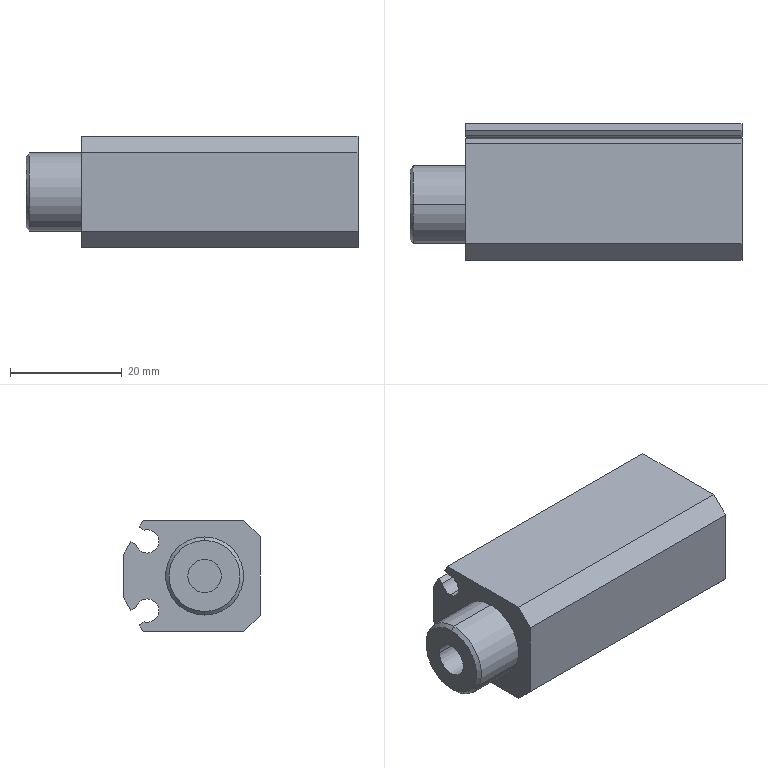Part | SolidWorks | features RefAxis 18, 3DProfileFeature 6, RevCut 3, Extrusion 1, Revolution 1 | 1 solid | 45 faces | box 59.5 x 24.5 x 20 mm | volume 16440 mm3 | plane 19 | cylinder 16 | cone 10 | commonest cylinder face diameters 4.2 x6 4.134 x4 6 x2 14 x2 16 x2
STEP:
#1=CARTESIAN_POINT('',(42.,7.258,0.));
#2=VERTEX_POINT('',#1);
#3=CARTESIAN_POINT('',(42.,8.5,2.067));
#4=VERTEX_POINT('',#3);
#5=CARTESIAN_POINT('',(42.,7.258,0.));
#6=DIRECTION('',(0.,0.515,0.8572));
#7=VECTOR('',#6,1000.);
#8=LINE('',#5,#7);
#9=EDGE_CURVE('',#2,#4,#8,.T.);
#10=ORIENTED_EDGE('',*,*,#9,.F.);
#11=CARTESIAN_POINT('',(42.,8.5,-2.067));
#12=VERTEX_POINT('',#11);
#13=CARTESIAN_POINT('',(42.,7.258,0.));
#14=DIRECTION('',(0.,0.515,-0.8572));
#15=VECTOR('',#14,1000.);
#16=LINE('',#13,#15);
#17=EDGE_CURVE('',#2,#12,#16,.T.);
#18=ORIENTED_EDGE('',*,*,#17,.T.);
#19=CARTESIAN_POINT('',(42.,8.5,0.));
#20=DIRECTION('',(0.,-1.,0.));
#21=DIRECTION('',(0.,0.,-1.));
#22=AXIS2_PLACEMENT_3D('',#19,#20,#21);
#23=CIRCLE('',#22,2.067);
#24=EDGE_CURVE('',#4,#12,#23,.T.);
#25=ORIENTED_EDGE('',*,*,#24,.F.);
#26=EDGE_LOOP('',(#10,#18,#25));
#27=FACE_OUTER_BOUND('',#26,.T.);
#28=CARTESIAN_POINT('',(42.,1007.258,0.));
#29=DIRECTION('',(0.,1.,0.));
#30=DIRECTION('',(0.,0.,1.));
#31=AXIS2_PLACEMENT_3D('',#28,#29,#30);
#32=CONICAL_SURFACE('',#31,1664.279,1.03);
#33=ADVANCED_FACE('',(#27),#32,.F.);
#34=CARTESIAN_POINT('',(42.,14.067,2.067));
#35=VERTEX_POINT('',#34);
#36=CARTESIAN_POINT('',(42.,14.067,-2.067));
#37=VERTEX_POINT('',#36);
#38=CARTESIAN_POINT('',(42.,14.067,0.));
#39=DIRECTION('',(0.,-1.,0.));
#40=DIRECTION('',(0.,0.,-1.));
#41=AXIS2_PLACEMENT_3D('',#38,#39,#40);
#42=CIRCLE('',#41,2.067);
#43=EDGE_CURVE('',#35,#37,#42,.T.);
#44=ORIENTED_EDGE('',*,*,#43,.F.);
#45=CARTESIAN_POINT('',(42.,7.258,2.067));
#46=DIRECTION('',(0.,-1.,0.));
#47=VECTOR('',#46,1000.);
#48=LINE('',#45,#47);
#49=EDGE_CURVE('',#35,#4,#48,.T.);
#50=ORIENTED_EDGE('',*,*,#49,.T.);
#51=ORIENTED_EDGE('',*,*,#24,.T.);
#52=CARTESIAN_POINT('',(42.,7.258,-2.067));
#53=DIRECTION('',(0.,-1.,0.));
#54=VECTOR('',#53,1000.);
#55=LINE('',#52,#54);
#56=EDGE_CURVE('',#37,#12,#55,.T.);
#57=ORIENTED_EDGE('',*,*,#56,.F.);
#58=EDGE_LOOP('',(#44,#50,#51,#57));
#59=FACE_OUTER_BOUND('',#58,.T.);
#60=CARTESIAN_POINT('',(42.,7.258,0.));
#61=DIRECTION('',(0.,-1.,0.));
#62=DIRECTION('',(0.,0.,-1.));
#63=AXIS2_PLACEMENT_3D('',#60,#61,#62);
#64=CYLINDRICAL_SURFACE('',#63,2.067);
#65=ADVANCED_FACE('',(#59),#64,.F.);
#66=ORIENTED_EDGE('',*,*,#43,.T.);
#67=CARTESIAN_POINT('',(42.,14.5,-2.5));
#68=VERTEX_POINT('',#67);
#69=CARTESIAN_POINT('',(42.,14.067,-2.067));
#70=DIRECTION('',(0.,0.7071,-0.7071));
#71=VECTOR('',#70,1000.);
#72=LINE('',#69,#71);
#73=EDGE_CURVE('',#37,#68,#72,.T.);
#74=ORIENTED_EDGE('',*,*,#73,.T.);
#75=CARTESIAN_POINT('',(42.,14.5,2.5));
#76=VERTEX_POINT('',#75);
#77=CARTESIAN_POINT('',(42.,14.5,0.));
#78=DIRECTION('',(0.,-1.,0.));
#79=DIRECTION('',(0.,0.,-1.));
#80=AXIS2_PLACEMENT_3D('',#77,#78,#79);
#81=CIRCLE('',#80,2.5);
#82=EDGE_CURVE('',#76,#68,#81,.T.);
#83=ORIENTED_EDGE('',*,*,#82,.F.);
#84=CARTESIAN_POINT('',(42.,14.067,2.067));
#85=DIRECTION('',(0.,0.7071,0.7071));
#86=VECTOR('',#85,1000.);
#87=LINE('',#84,#86);
#88=EDGE_CURVE('',#35,#76,#87,.T.);
#89=ORIENTED_EDGE('',*,*,#88,.F.);
#90=EDGE_LOOP('',(#66,#74,#83,#89));
#91=FACE_OUTER_BOUND('',#90,.T.);
#92=CARTESIAN_POINT('',(42.,14.067,0.));
#93=DIRECTION('',(0.,1.,0.));
#94=DIRECTION('',(0.,0.,1.));
#95=AXIS2_PLACEMENT_3D('',#92,#93,#94);
#96=CONICAL_SURFACE('',#95,2.067,0.7854);
#97=ADVANCED_FACE('',(#91),#96,.F.);
#98=CARTESIAN_POINT('',(6.5,7.258,0.));
#99=VERTEX_POINT('',#98);
#100=CARTESIAN_POINT('',(6.5,8.5,2.067));
#101=VERTEX_POINT('',#100);
#102=CARTESIAN_POINT('',(6.5,7.258,0.));
#103=DIRECTION('',(0.,0.515,0.8572));
#104=VECTOR('',#103,1000.);
#105=LINE('',#102,#104);
#106=EDGE_CURVE('',#99,#101,#105,.T.);
#107=ORIENTED_EDGE('',*,*,#106,.F.);
#108=CARTESIAN_POINT('',(6.5,8.5,-2.067));
#109=VERTEX_POINT('',#108);
#110=CARTESIAN_POINT('',(6.5,7.258,0.));
#111=DIRECTION('',(0.,0.515,-0.8572));
#112=VECTOR('',#111,1000.);
#113=LINE('',#110,#112);
#114=EDGE_CURVE('',#99,#109,#113,.T.);
#115=ORIENTED_EDGE('',*,*,#114,.T.);
#116=CARTESIAN_POINT('',(6.5,8.5,0.));
#117=DIRECTION('',(0.,-1.,0.));
#118=DIRECTION('',(0.,0.,-1.));
#119=AXIS2_PLACEMENT_3D('',#116,#117,#118);
#120=CIRCLE('',#119,2.067);
#121=EDGE_CURVE('',#101,#109,#120,.T.);
#122=ORIENTED_EDGE('',*,*,#121,.F.);
#123=EDGE_LOOP('',(#107,#115,#122));
#124=FACE_OUTER_BOUND('',#123,.T.);
#125=CARTESIAN_POINT('',(6.5,1007.258,0.));
#126=DIRECTION('',(0.,1.,0.));
#127=DIRECTION('',(0.,0.,1.));
#128=AXIS2_PLACEMENT_3D('',#125,#126,#127);
#129=CONICAL_SURFACE('',#128,1664.279,1.03);
#130=ADVANCED_FACE('',(#124),#129,.F.);
#131=CARTESIAN_POINT('',(6.5,14.067,2.067));
#132=VERTEX_POINT('',#131);
#133=CARTESIAN_POINT('',(6.5,14.067,-2.067));
#134=VERTEX_POINT('',#133);
#135=CARTESIAN_POINT('',(6.5,14.067,0.));
#136=DIRECTION('',(0.,-1.,0.));
#137=DIRECTION('',(0.,0.,-1.));
#138=AXIS2_PLACEMENT_3D('',#135,#136,#137);
#139=CIRCLE('',#138,2.067);
#140=EDGE_CURVE('',#132,#134,#139,.T.);
#141=ORIENTED_EDGE('',*,*,#140,.F.);
#142=CARTESIAN_POINT('',(6.5,7.258,2.067));
#143=DIRECTION('',(0.,-1.,0.));
#144=VECTOR('',#143,1000.);
#145=LINE('',#142,#144);
#146=EDGE_CURVE('',#132,#101,#145,.T.);
#147=ORIENTED_EDGE('',*,*,#146,.T.);
#148=ORIENTED_EDGE('',*,*,#121,.T.);
#149=CARTESIAN_POINT('',(6.5,7.258,-2.067));
#150=DIRECTION('',(0.,-1.,0.));
#151=VECTOR('',#150,1000.);
#152=LINE('',#149,#151);
#153=EDGE_CURVE('',#134,#109,#152,.T.);
#154=ORIENTED_EDGE('',*,*,#153,.F.);
#155=EDGE_LOOP('',(#141,#147,#148,#154));
#156=FACE_OUTER_BOUND('',#155,.T.);
#157=CARTESIAN_POINT('',(6.5,7.258,0.));
#158=DIRECTION('',(0.,-1.,0.));
#159=DIRECTION('',(0.,0.,-1.));
#160=AXIS2_PLACEMENT_3D('',#157,#158,#159);
#161=CYLINDRICAL_SURFACE('',#160,2.067);
#162=ADVANCED_FACE('',(#156),#161,.F.);
#163=ORIENTED_EDGE('',*,*,#140,.T.);
#164=CARTESIAN_POINT('',(6.5,14.5,-2.5));
#165=VERTEX_POINT('',#164);
#166=CARTESIAN_POINT('',(6.5,14.067,-2.067));
#167=DIRECTION('',(0.,0.7071,-0.7071));
#168=VECTOR('',#167,1000.);
#169=LINE('',#166,#168);
#170=EDGE_CURVE('',#134,#165,#169,.T.);
#171=ORIENTED_EDGE('',*,*,#170,.T.);
#172=CARTESIAN_POINT('',(6.5,14.5,2.5));
#173=VERTEX_POINT('',#172);
#174=CARTESIAN_POINT('',(6.5,14.5,0.));
#175=DIRECTION('',(0.,-1.,0.));
#176=DIRECTION('',(0.,0.,-1.));
#177=AXIS2_PLACEMENT_3D('',#174,#175,#176);
#178=CIRCLE('',#177,2.5);
#179=EDGE_CURVE('',#173,#165,#178,.T.);
#180=ORIENTED_EDGE('',*,*,#179,.F.);
#181=CARTESIAN_POINT('',(6.5,14.067,2.067));
#182=DIRECTION('',(0.,0.7071,0.7071));
#183=VECTOR('',#182,1000.);
#184=LINE('',#181,#183);
#185=EDGE_CURVE('',#132,#173,#184,.T.);
#186=ORIENTED_EDGE('',*,*,#185,.F.);
#187=EDGE_LOOP('',(#163,#171,#180,#186));
#188=FACE_OUTER_BOUND('',#187,.T.);
#189=CARTESIAN_POINT('',(6.5,14.067,0.));
#190=DIRECTION('',(0.,1.,0.));
#191=DIRECTION('',(0.,0.,1.));
#192=AXIS2_PLACEMENT_3D('',#189,#190,#191);
#193=CONICAL_SURFACE('',#192,2.067,0.7854);
#194=ADVANCED_FACE('',(#188),#193,.F.);
#195=CARTESIAN_POINT('',(11.,-8.,0.));
#196=VERTEX_POINT('',#195);
#197=CARTESIAN_POINT('',(11.,8.,0.));
#198=VERTEX_POINT('',#197);
#199=CARTESIAN_POINT('',(11.,0.,0.));
#200=DIRECTION('',(1.,0.,0.));
#201=DIRECTION('',(0.,1.,0.));
#202=AXIS2_PLACEMENT_3D('',#199,#200,#201);
#203=CIRCLE('',#202,8.);
#204=EDGE_CURVE('',#196,#198,#203,.T.);
#205=ORIENTED_EDGE('',*,*,#204,.F.);
#206=CARTESIAN_POINT('',(38.5,-8.,0.));
#207=VERTEX_POINT('',#206);
#208=CARTESIAN_POINT('',(38.5,-8.,0.));
#209=DIRECTION('',(1.,0.,0.));
#210=VECTOR('',#209,1000.);
#211=LINE('',#208,#210);
#212=EDGE_CURVE('',#196,#207,#211,.T.);
#213=ORIENTED_EDGE('',*,*,#212,.T.);
#214=CARTESIAN_POINT('',(38.5,8.,0.));
#215=VERTEX_POINT('',#214);
#216=CARTESIAN_POINT('',(38.5,0.,0.));
#217=DIRECTION('',(1.,0.,0.));
#218=DIRECTION('',(0.,1.,0.));
#219=AXIS2_PLACEMENT_3D('',#216,#217,#218);
#220=CIRCLE('',#219,8.);
#221=EDGE_CURVE('',#207,#215,#220,.T.);
#222=ORIENTED_EDGE('',*,*,#221,.T.);
#223=CARTESIAN_POINT('',(38.5,8.,0.));
#224=DIRECTION('',(1.,0.,0.));
#225=VECTOR('',#224,1000.);
#226=LINE('',#223,#225);
#227=EDGE_CURVE('',#198,#215,#226,.T.);
#228=ORIENTED_EDGE('',*,*,#227,.F.);
#229=EDGE_LOOP('',(#205,#213,#222,#228));
#230=FACE_OUTER_BOUND('',#229,.T.);
#231=CARTESIAN_POINT('',(38.5,0.,0.));
#232=DIRECTION('',(1.,0.,0.));
#233=DIRECTION('',(0.,1.,0.));
#234=AXIS2_PLACEMENT_3D('',#231,#232,#233);
#235=CYLINDRICAL_SURFACE('',#234,8.);
#236=ADVANCED_FACE('',(#230),#235,.F.);
#237=CARTESIAN_POINT('',(-10.,-3.,0.));
#238=VERTEX_POINT('',#237);
#239=CARTESIAN_POINT('',(-10.,3.,0.));
#240=VERTEX_POINT('',#239);
#241=CARTESIAN_POINT('',(-10.,0.,0.));
#242=DIRECTION('',(1.,0.,0.));
#243=DIRECTION('',(0.,1.,0.));
#244=AXIS2_PLACEMENT_3D('',#241,#242,#243);
#245=CIRCLE('',#244,3.);
#246=EDGE_CURVE('',#238,#240,#245,.T.);
#247=ORIENTED_EDGE('',*,*,#246,.F.);
#248=CARTESIAN_POINT('',(11.,-3.,0.));
#249=VERTEX_POINT('',#248);
#250=CARTESIAN_POINT('',(38.5,-3.,0.));
#251=DIRECTION('',(1.,0.,0.));
#252=VECTOR('',#251,1000.);
#253=LINE('',#250,#252);
#254=EDGE_CURVE('',#238,#249,#253,.T.);
#255=ORIENTED_EDGE('',*,*,#254,.T.);
#256=CARTESIAN_POINT('',(11.,3.,0.));
#257=VERTEX_POINT('',#256);
#258=CARTESIAN_POINT('',(11.,0.,0.));
#259=DIRECTION('',(1.,0.,0.));
#260=DIRECTION('',(0.,1.,0.));
#261=AXIS2_PLACEMENT_3D('',#258,#259,#260);
#262=CIRCLE('',#261,3.);
#263=EDGE_CURVE('',#249,#257,#262,.T.);
#264=ORIENTED_EDGE('',*,*,#263,.T.);
#265=CARTESIAN_POINT('',(38.5,3.,0.));
#266=DIRECTION('',(1.,0.,0.));
#267=VECTOR('',#266,1000.);
#268=LINE('',#265,#267);
#269=EDGE_CURVE('',#240,#257,#268,.T.);
#270=ORIENTED_EDGE('',*,*,#269,.F.);
#271=EDGE_LOOP('',(#247,#255,#264,#270));
#272=FACE_OUTER_BOUND('',#271,.T.);
#273=CARTESIAN_POINT('',(38.5,0.,0.));
#274=DIRECTION('',(1.,0.,0.));
#275=DIRECTION('',(0.,1.,0.));
#276=AXIS2_PLACEMENT_3D('',#273,#274,#275);
#277=CYLINDRICAL_SURFACE('',#276,3.);
#278=ADVANCED_FACE('',(#272),#277,.F.);
#279=CARTESIAN_POINT('',(-9.386,0.,-7.));
#280=VERTEX_POINT('',#279);
#281=CARTESIAN_POINT('',(-9.386,0.,7.));
#282=VERTEX_POINT('',#281);
#283=CARTESIAN_POINT('',(-9.386,0.,0.));
#284=DIRECTION('',(1.,0.,0.));
#285=DIRECTION('',(0.,0.,-1.));
#286=AXIS2_PLACEMENT_3D('',#283,#284,#285);
#287=CIRCLE('',#286,7.);
#288=EDGE_CURVE('',#280,#282,#287,.T.);
#289=ORIENTED_EDGE('',*,*,#288,.T.);
#290=CARTESIAN_POINT('',(0.,0.,7.));
#291=VERTEX_POINT('',#290);
#292=CARTESIAN_POINT('',(0.,0.,7.));
#293=DIRECTION('',(1.,0.,0.));
#294=VECTOR('',#293,1000.);
#295=LINE('',#292,#294);
#296=EDGE_CURVE('',#282,#291,#295,.T.);
#297=ORIENTED_EDGE('',*,*,#296,.T.);
#298=CARTESIAN_POINT('',(0.,0.,-7.));
#299=VERTEX_POINT('',#298);
#300=CARTESIAN_POINT('',(0.,0.,0.));
#301=DIRECTION('',(-1.,0.,0.));
#302=DIRECTION('',(0.,0.,1.));
#303=AXIS2_PLACEMENT_3D('',#300,#301,#302);
#304=CIRCLE('',#303,7.);
#305=EDGE_CURVE('',#291,#299,#304,.T.);
#306=ORIENTED_EDGE('',*,*,#305,.T.);
#307=CARTESIAN_POINT('',(0.,0.,-7.));
#308=DIRECTION('',(1.,0.,0.));
#309=VECTOR('',#308,1000.);
#310=LINE('',#307,#309);
#311=EDGE_CURVE('',#280,#299,#310,.T.);
#312=ORIENTED_EDGE('',*,*,#311,.F.);
#313=EDGE_LOOP('',(#289,#297,#306,#312));
#314=FACE_OUTER_BOUND('',#313,.T.);
#315=CARTESIAN_POINT('',(0.,0.,0.));
#316=DIRECTION('',(1.,0.,0.));
#317=DIRECTION('',(0.,0.,-1.));
#318=AXIS2_PLACEMENT_3D('',#315,#316,#317);
#319=CYLINDRICAL_SURFACE('',#318,7.);
#320=ADVANCED_FACE('',(#314),#319,.T.);
#321=CARTESIAN_POINT('',(-10.,0.,-6.386));
#322=VERTEX_POINT('',#321);
#323=CARTESIAN_POINT('',(-10.,0.,6.386));
#324=VERTEX_POINT('',#323);
#325=CARTESIAN_POINT('',(-10.,0.,0.));
#326=DIRECTION('',(1.,0.,0.));
#327=DIRECTION('',(0.,0.,-1.));
#328=AXIS2_PLACEMENT_3D('',#325,#326,#327);
#329=CIRCLE('',#328,6.386);
#330=EDGE_CURVE('',#322,#324,#329,.T.);
#331=ORIENTED_EDGE('',*,*,#330,.T.);
#332=CARTESIAN_POINT('',(-9.386,0.,7.));
#333=DIRECTION('',(0.7071,0.,0.7071));
#334=VECTOR('',#333,1000.);
#335=LINE('',#332,#334);
#336=EDGE_CURVE('',#324,#282,#335,.T.);
#337=ORIENTED_EDGE('',*,*,#336,.T.);
#338=ORIENTED_EDGE('',*,*,#288,.F.);
#339=CARTESIAN_POINT('',(-9.386,0.,-7.));
#340=DIRECTION('',(0.7071,0.,-0.7071));
#341=VECTOR('',#340,1000.);
#342=LINE('',#339,#341);
#343=EDGE_CURVE('',#322,#280,#342,.T.);
#344=ORIENTED_EDGE('',*,*,#343,.F.);
#345=EDGE_LOOP('',(#331,#337,#338,#344));
#346=FACE_OUTER_BOUND('',#345,.T.);
#347=CARTESIAN_POINT('',(-9.386,0.,0.));
#348=DIRECTION('',(1.,0.,0.));
#349=DIRECTION('',(0.,0.,-1.));
#350=AXIS2_PLACEMENT_3D('',#347,#348,#349);
#351=CONICAL_SURFACE('',#350,7.,0.7854);
#352=ADVANCED_FACE('',(#346),#351,.T.);
#353=CARTESIAN_POINT('',(49.5,10.3,4.1));
#354=VERTEX_POINT('',#353);
#355=CARTESIAN_POINT('',(49.5,10.3,8.3));
#356=VERTEX_POINT('',#355);
#357=CARTESIAN_POINT('',(49.5,10.3,6.2));
#358=DIRECTION('',(-1.,0.,0.));
#359=DIRECTION('',(0.,0.,1.));
#360=AXIS2_PLACEMENT_3D('',#357,#358,#359);
#361=CIRCLE('',#360,2.1);
#362=EDGE_CURVE('',#354,#356,#361,.T.);
#363=ORIENTED_EDGE('',*,*,#362,.F.);
#364=CARTESIAN_POINT('',(0.,10.3,4.1));
#365=VERTEX_POINT('',#364);
#366=CARTESIAN_POINT('',(49.5,10.3,4.1));
#367=DIRECTION('',(-1.,0.,0.));
#368=VECTOR('',#367,1000.);
#369=LINE('',#366,#368);
#370=EDGE_CURVE('',#354,#365,#369,.T.);
#371=ORIENTED_EDGE('',*,*,#370,.T.);
#372=CARTESIAN_POINT('',(0.,10.3,8.3));
#373=VERTEX_POINT('',#372);
#374=CARTESIAN_POINT('',(0.,10.3,6.2));
#375=DIRECTION('',(-1.,0.,0.));
#376=DIRECTION('',(0.,0.,1.));
#377=AXIS2_PLACEMENT_3D('',#374,#375,#376);
#378=CIRCLE('',#377,2.1);
#379=EDGE_CURVE('',#365,#373,#378,.T.);
#380=ORIENTED_EDGE('',*,*,#379,.T.);
#381=CARTESIAN_POINT('',(49.5,10.3,8.3));
#382=DIRECTION('',(-1.,0.,0.));
#383=VECTOR('',#382,1000.);
#384=LINE('',#381,#383);
#385=EDGE_CURVE('',#356,#373,#384,.T.);
#386=ORIENTED_EDGE('',*,*,#385,.F.);
#387=EDGE_LOOP('',(#363,#371,#380,#386));
#388=FACE_OUTER_BOUND('',#387,.T.);
#389=CARTESIAN_POINT('',(49.5,10.3,6.2));
#390=DIRECTION('',(-1.,0.,0.));
#391=DIRECTION('',(0.,0.,1.));
#392=AXIS2_PLACEMENT_3D('',#389,#390,#391);
#393=CYLINDRICAL_SURFACE('',#392,2.1);
#394=ADVANCED_FACE('',(#388),#393,.F.);
#395=CARTESIAN_POINT('',(49.5,10.823,8.234));
#396=VERTEX_POINT('',#395);
#397=CARTESIAN_POINT('',(49.5,10.3,6.2));
#398=DIRECTION('',(-1.,0.,0.));
#399=DIRECTION('',(0.,0.,1.));
#400=AXIS2_PLACEMENT_3D('',#397,#398,#399);
#401=CIRCLE('',#400,2.1);
#402=EDGE_CURVE('',#356,#396,#401,.T.);
#403=ORIENTED_EDGE('',*,*,#402,.F.);
#404=ORIENTED_EDGE('',*,*,#385,.T.);
#405=CARTESIAN_POINT('',(0.,10.823,8.234));
#406=VERTEX_POINT('',#405);
#407=CARTESIAN_POINT('',(0.,10.3,6.2));
#408=DIRECTION('',(-1.,0.,0.));
#409=DIRECTION('',(0.,0.,1.));
#410=AXIS2_PLACEMENT_3D('',#407,#408,#409);
#411=CIRCLE('',#410,2.1);
#412=EDGE_CURVE('',#373,#406,#411,.T.);
#413=ORIENTED_EDGE('',*,*,#412,.T.);
#414=CARTESIAN_POINT('',(49.5,10.823,8.234));
#415=DIRECTION('',(-1.,0.,0.));
#416=VECTOR('',#415,1000.);
#417=LINE('',#414,#416);
#418=EDGE_CURVE('',#396,#406,#417,.T.);
#419=ORIENTED_EDGE('',*,*,#418,.F.);
#420=EDGE_LOOP('',(#403,#404,#413,#419));
#421=FACE_OUTER_BOUND('',#420,.T.);
#422=CARTESIAN_POINT('',(49.5,10.3,6.2));
#423=DIRECTION('',(-1.,0.,0.));
#424=DIRECTION('',(0.,0.,1.));
#425=AXIS2_PLACEMENT_3D('',#422,#423,#424);
#426=CYLINDRICAL_SURFACE('',#425,2.1);
#427=ADVANCED_FACE('',(#421),#426,.F.);
#428=CARTESIAN_POINT('',(49.5,10.3,-8.3));
#429=VERTEX_POINT('',#428);
#430=CARTESIAN_POINT('',(49.5,10.3,-4.1));
#431=VERTEX_POINT('',#430);
#432=CARTESIAN_POINT('',(49.5,10.3,-6.2));
#433=DIRECTION('',(-1.,0.,0.));
#434=DIRECTION('',(0.,0.,1.));
#435=AXIS2_PLACEMENT_3D('',#432,#433,#434);
#436=CIRCLE('',#435,2.1);
#437=EDGE_CURVE('',#429,#431,#436,.T.);
#438=ORIENTED_EDGE('',*,*,#437,.F.);
#439=CARTESIAN_POINT('',(0.,10.3,-8.3));
#440=VERTEX_POINT('',#439);
#441=CARTESIAN_POINT('',(49.5,10.3,-8.3));
#442=DIRECTION('',(-1.,0.,0.));
#443=VECTOR('',#442,1000.);
#444=LINE('',#441,#443);
#445=EDGE_CURVE('',#429,#440,#444,.T.);
#446=ORIENTED_EDGE('',*,*,#445,.T.);
#447=CARTESIAN_POINT('',(0.,10.3,-4.1));
#448=VERTEX_POINT('',#447);
#449=CARTESIAN_POINT('',(0.,10.3,-6.2));
#450=DIRECTION('',(-1.,0.,0.));
#451=DIRECTION('',(0.,0.,1.));
#452=AXIS2_PLACEMENT_3D('',#449,#450,#451);
#453=CIRCLE('',#452,2.1);
#454=EDGE_CURVE('',#440,#448,#453,.T.);
#455=ORIENTED_EDGE('',*,*,#454,.T.);
#456=CARTESIAN_POINT('',(49.5,10.3,-4.1));
#457=DIRECTION('',(-1.,0.,0.));
#458=VECTOR('',#457,1000.);
#459=LINE('',#456,#458);
#460=EDGE_CURVE('',#431,#448,#459,.T.);
#461=ORIENTED_EDGE('',*,*,#460,.F.);
#462=EDGE_LOOP('',(#438,#446,#455,#461));
#463=FACE_OUTER_BOUND('',#462,.T.);
#464=CARTESIAN_POINT('',(49.5,10.3,-6.2));
#465=DIRECTION('',(-1.,0.,0.));
#466=DIRECTION('',(0.,0.,1.));
#467=AXIS2_PLACEMENT_3D('',#464,#465,#466);
#468=CYLINDRICAL_SURFACE('',#467,2.1);
#469=ADVANCED_FACE('',(#463),#468,.F.);
#470=CARTESIAN_POINT('',(49.5,12.323,-5.636));
#471=VERTEX_POINT('',#470);
#472=CARTESIAN_POINT('',(49.5,10.3,-6.2));
#473=DIRECTION('',(-1.,0.,0.));
#474=DIRECTION('',(0.,0.,1.));
#475=AXIS2_PLACEMENT_3D('',#472,#473,#474);
#476=CIRCLE('',#475,2.1);
#477=EDGE_CURVE('',#431,#471,#476,.T.);
#478=ORIENTED_EDGE('',*,*,#477,.F.);
#479=ORIENTED_EDGE('',*,*,#460,.T.);
#480=CARTESIAN_POINT('',(0.,12.323,-5.636));
#481=VERTEX_POINT('',#480);
#482=CARTESIAN_POINT('',(0.,10.3,-6.2));
#483=DIRECTION('',(-1.,0.,0.));
#484=DIRECTION('',(0.,0.,1.));
#485=AXIS2_PLACEMENT_3D('',#482,#483,#484);
#486=CIRCLE('',#485,2.1);
#487=EDGE_CURVE('',#448,#481,#486,.T.);
#488=ORIENTED_EDGE('',*,*,#487,.T.);
#489=CARTESIAN_POINT('',(49.5,12.323,-5.636));
#490=DIRECTION('',(-1.,0.,0.));
#491=VECTOR('',#490,1000.);
#492=LINE('',#489,#491);
#493=EDGE_CURVE('',#471,#481,#492,.T.);
#494=ORIENTED_EDGE('',*,*,#493,.F.);
#495=EDGE_LOOP('',(#478,#479,#488,#494));
#496=FACE_OUTER_BOUND('',#495,.T.);
#497=CARTESIAN_POINT('',(49.5,10.3,-6.2));
#498=DIRECTION('',(-1.,0.,0.));
#499=DIRECTION('',(0.,0.,1.));
#500=AXIS2_PLACEMENT_3D('',#497,#498,#499);
#501=CYLINDRICAL_SURFACE('',#500,2.1);
#502=ADVANCED_FACE('',(#496),#501,.F.);
#503=CARTESIAN_POINT('',(0.,10.993,10.));
#504=VERTEX_POINT('',#503);
#505=CARTESIAN_POINT('',(0.,-7.,10.));
#506=VERTEX_POINT('',#505);
#507=CARTESIAN_POINT('',(0.,10.993,10.));
#508=DIRECTION('',(0.,-1.,0.));
#509=VECTOR('',#508,1000.);
#510=LINE('',#507,#509);
#511=EDGE_CURVE('',#504,#506,#510,.T.);
#512=ORIENTED_EDGE('',*,*,#511,.T.);
#513=CARTESIAN_POINT('',(49.5,-7.,10.));
#514=VERTEX_POINT('',#513);
#515=CARTESIAN_POINT('',(49.5,-7.,10.));
#516=DIRECTION('',(-1.,0.,0.));
#517=VECTOR('',#516,1000.);
#518=LINE('',#515,#517);
#519=EDGE_CURVE('',#514,#506,#518,.T.);
#520=ORIENTED_EDGE('',*,*,#519,.F.);
#521=CARTESIAN_POINT('',(49.5,10.993,10.));
#522=VERTEX_POINT('',#521);
#523=CARTESIAN_POINT('',(49.5,10.993,10.));
#524=DIRECTION('',(0.,-1.,0.));
#525=VECTOR('',#524,1000.);
#526=LINE('',#523,#525);
#527=EDGE_CURVE('',#522,#514,#526,.T.);
#528=ORIENTED_EDGE('',*,*,#527,.F.);
#529=CARTESIAN_POINT('',(49.5,10.993,10.));
#530=DIRECTION('',(-1.,0.,0.));
#531=VECTOR('',#530,1000.);
#532=LINE('',#529,#531);
#533=EDGE_CURVE('',#522,#504,#532,.T.);
#534=ORIENTED_EDGE('',*,*,#533,.T.);
#535=EDGE_LOOP('',(#512,#520,#528,#534));
#536=FACE_OUTER_BOUND('',#535,.T.);
#537=CARTESIAN_POINT('',(49.5,10.993,10.));
#538=DIRECTION('',(0.,0.,-1.));
#539=DIRECTION('',(-1.,0.,0.));
#540=AXIS2_PLACEMENT_3D('',#537,#538,#539);
#541=PLANE('',#540);
#542=ADVANCED_FACE('',(#536),#541,.F.);
#543=CARTESIAN_POINT('',(0.,-10.,7.));
#544=VERTEX_POINT('',#543);
#545=CARTESIAN_POINT('',(0.,-7.,10.));
#546=DIRECTION('',(0.,-0.7071,-0.7071));
#547=VECTOR('',#546,1000.);
#548=LINE('',#545,#547);
#549=EDGE_CURVE('',#506,#544,#548,.T.);
#550=ORIENTED_EDGE('',*,*,#549,.T.);
#551=CARTESIAN_POINT('',(49.5,-10.,7.));
#552=VERTEX_POINT('',#551);
#553=CARTESIAN_POINT('',(49.5,-10.,7.));
#554=DIRECTION('',(-1.,0.,0.));
#555=VECTOR('',#554,1000.);
#556=LINE('',#553,#555);
#557=EDGE_CURVE('',#552,#544,#556,.T.);
#558=ORIENTED_EDGE('',*,*,#557,.F.);
#559=CARTESIAN_POINT('',(49.5,-7.,10.));
#560=DIRECTION('',(0.,-0.7071,-0.7071));
#561=VECTOR('',#560,1000.);
#562=LINE('',#559,#561);
#563=EDGE_CURVE('',#514,#552,#562,.T.);
#564=ORIENTED_EDGE('',*,*,#563,.F.);
#565=ORIENTED_EDGE('',*,*,#519,.T.);
#566=EDGE_LOOP('',(#550,#558,#564,#565));
#567=FACE_OUTER_BOUND('',#566,.T.);
#568=CARTESIAN_POINT('',(49.5,-7.,10.));
#569=DIRECTION('',(0.,0.7071,-0.7071));
#570=DIRECTION('',(0.,0.7071,0.7071));
#571=AXIS2_PLACEMENT_3D('',#568,#569,#570);
#572=PLANE('',#571);
#573=ADVANCED_FACE('',(#567),#572,.F.);
#574=CARTESIAN_POINT('',(0.,-10.,-7.));
#575=VERTEX_POINT('',#574);
#576=CARTESIAN_POINT('',(0.,-10.,7.));
#577=DIRECTION('',(0.,0.,-1.));
#578=VECTOR('',#577,1000.);
#579=LINE('',#576,#578);
#580=EDGE_CURVE('',#544,#575,#579,.T.);
#581=ORIENTED_EDGE('',*,*,#580,.T.);
#582=CARTESIAN_POINT('',(49.5,-10.,-7.));
#583=VERTEX_POINT('',#582);
#584=CARTESIAN_POINT('',(49.5,-10.,-7.));
#585=DIRECTION('',(-1.,0.,0.));
#586=VECTOR('',#585,1000.);
#587=LINE('',#584,#586);
#588=EDGE_CURVE('',#583,#575,#587,.T.);
#589=ORIENTED_EDGE('',*,*,#588,.F.);
#590=CARTESIAN_POINT('',(49.5,-10.,7.));
#591=DIRECTION('',(0.,0.,-1.));
#592=VECTOR('',#591,1000.);
#593=LINE('',#590,#592);
#594=EDGE_CURVE('',#552,#583,#593,.T.);
#595=ORIENTED_EDGE('',*,*,#594,.F.);
#596=ORIENTED_EDGE('',*,*,#557,.T.);
#597=EDGE_LOOP('',(#581,#589,#595,#596));
#598=FACE_OUTER_BOUND('',#597,.T.);
#599=CARTESIAN_POINT('',(49.5,-10.,7.));
#600=DIRECTION('',(0.,1.,0.));
#601=DIRECTION('',(0.,0.,1.));
#602=AXIS2_PLACEMENT_3D('',#599,#600,#601);
#603=PLANE('',#602);
#604=ADVANCED_FACE('',(#598),#603,.F.);
#605=CARTESIAN_POINT('',(0.,-7.,-10.));
#606=VERTEX_POINT('',#605);
#607=CARTESIAN_POINT('',(0.,-10.,-7.));
#608=DIRECTION('',(0.,0.7071,-0.7071));
#609=VECTOR('',#608,1000.);
#610=LINE('',#607,#609);
#611=EDGE_CURVE('',#575,#606,#610,.T.);
#612=ORIENTED_EDGE('',*,*,#611,.T.);
#613=CARTESIAN_POINT('',(49.5,-7.,-10.));
#614=VERTEX_POINT('',#613);
#615=CARTESIAN_POINT('',(49.5,-7.,-10.));
#616=DIRECTION('',(-1.,0.,0.));
#617=VECTOR('',#616,1000.);
#618=LINE('',#615,#617);
#619=EDGE_CURVE('',#614,#606,#618,.T.);
#620=ORIENTED_EDGE('',*,*,#619,.F.);
#621=CARTESIAN_POINT('',(49.5,-10.,-7.));
#622=DIRECTION('',(0.,0.7071,-0.7071));
#623=VECTOR('',#622,1000.);
#624=LINE('',#621,#623);
#625=EDGE_CURVE('',#583,#614,#624,.T.);
#626=ORIENTED_EDGE('',*,*,#625,.F.);
#627=ORIENTED_EDGE('',*,*,#588,.T.);
#628=EDGE_LOOP('',(#612,#620,#626,#627));
#629=FACE_OUTER_BOUND('',#628,.T.);
#630=CARTESIAN_POINT('',(49.5,-10.,-7.));
#631=DIRECTION('',(0.,0.7071,0.7071));
#632=DIRECTION('',(0.,-0.7071,0.7071));
#633=AXIS2_PLACEMENT_3D('',#630,#631,#632);
#634=PLANE('',#633);
#635=ADVANCED_FACE('',(#629),#634,.F.);
#636=CARTESIAN_POINT('',(0.,10.993,-10.));
#637=VERTEX_POINT('',#636);
#638=CARTESIAN_POINT('',(0.,-7.,-10.));
#639=DIRECTION('',(0.,1.,0.));
#640=VECTOR('',#639,1000.);
#641=LINE('',#638,#640);
#642=EDGE_CURVE('',#606,#637,#641,.T.);
#643=ORIENTED_EDGE('',*,*,#642,.T.);
#644=CARTESIAN_POINT('',(49.5,10.993,-10.));
#645=VERTEX_POINT('',#644);
#646=CARTESIAN_POINT('',(49.5,10.993,-10.));
#647=DIRECTION('',(-1.,0.,0.));
#648=VECTOR('',#647,1000.);
#649=LINE('',#646,#648);
#650=EDGE_CURVE('',#645,#637,#649,.T.);
#651=ORIENTED_EDGE('',*,*,#650,.F.);
#652=CARTESIAN_POINT('',(49.5,-7.,-10.));
#653=DIRECTION('',(0.,1.,0.));
#654=VECTOR('',#653,1000.);
#655=LINE('',#652,#654);
#656=EDGE_CURVE('',#614,#645,#655,.T.);
#657=ORIENTED_EDGE('',*,*,#656,.F.);
#658=ORIENTED_EDGE('',*,*,#619,.T.);
#659=EDGE_LOOP('',(#643,#651,#657,#658));
#660=FACE_OUTER_BOUND('',#659,.T.);
#661=CARTESIAN_POINT('',(49.5,-7.,-10.));
#662=DIRECTION('',(0.,0.,1.));
#663=DIRECTION('',(1.,0.,0.));
#664=AXIS2_PLACEMENT_3D('',#661,#662,#663);
#665=PLANE('',#664);
#666=ADVANCED_FACE('',(#660),#665,.F.);
#667=CARTESIAN_POINT('',(0.,11.715,-8.749));
#668=VERTEX_POINT('',#667);
#669=CARTESIAN_POINT('',(0.,10.993,-10.));
#670=DIRECTION('',(0.,0.5,0.866));
#671=VECTOR('',#670,1000.);
#672=LINE('',#669,#671);
#673=EDGE_CURVE('',#637,#668,#672,.T.);
#674=ORIENTED_EDGE('',*,*,#673,.T.);
#675=CARTESIAN_POINT('',(49.5,11.715,-8.749));
#676=VERTEX_POINT('',#675);
#677=CARTESIAN_POINT('',(49.5,11.715,-8.749));
#678=DIRECTION('',(-1.,0.,0.));
#679=VECTOR('',#678,1000.);
#680=LINE('',#677,#679);
#681=EDGE_CURVE('',#676,#668,#680,.T.);
#682=ORIENTED_EDGE('',*,*,#681,.F.);
#683=CARTESIAN_POINT('',(49.5,10.993,-10.));
#684=DIRECTION('',(0.,0.5,0.866));
#685=VECTOR('',#684,1000.);
#686=LINE('',#683,#685);
#687=EDGE_CURVE('',#645,#676,#686,.T.);
#688=ORIENTED_EDGE('',*,*,#687,.F.);
#689=ORIENTED_EDGE('',*,*,#650,.T.);
#690=EDGE_LOOP('',(#674,#682,#688,#689));
#691=FACE_OUTER_BOUND('',#690,.T.);
#692=CARTESIAN_POINT('',(49.5,10.993,-10.));
#693=DIRECTION('',(0.,-0.866,0.5));
#694=DIRECTION('',(0.,-0.5,-0.866));
#695=AXIS2_PLACEMENT_3D('',#692,#693,#694);
#696=PLANE('',#695);
#697=ADVANCED_FACE('',(#691),#696,.F.);
#698=CARTESIAN_POINT('',(0.,10.823,-8.234));
#699=VERTEX_POINT('',#698);
#700=CARTESIAN_POINT('',(0.,11.715,-8.749));
#701=DIRECTION('',(0.,-0.866,0.5));
#702=VECTOR('',#701,1000.);
#703=LINE('',#700,#702);
#704=EDGE_CURVE('',#668,#699,#703,.T.);
#705=ORIENTED_EDGE('',*,*,#704,.T.);
#706=CARTESIAN_POINT('',(49.5,10.823,-8.234));
#707=VERTEX_POINT('',#706);
#708=CARTESIAN_POINT('',(49.5,10.823,-8.234));
#709=DIRECTION('',(-1.,0.,0.));
#710=VECTOR('',#709,1000.);
#711=LINE('',#708,#710);
#712=EDGE_CURVE('',#707,#699,#711,.T.);
#713=ORIENTED_EDGE('',*,*,#712,.F.);
#714=CARTESIAN_POINT('',(49.5,11.715,-8.749));
#715=DIRECTION('',(0.,-0.866,0.5));
#716=VECTOR('',#715,1000.);
#717=LINE('',#714,#716);
#718=EDGE_CURVE('',#676,#707,#717,.T.);
#719=ORIENTED_EDGE('',*,*,#718,.F.);
#720=ORIENTED_EDGE('',*,*,#681,.T.);
#721=EDGE_LOOP('',(#705,#713,#719,#720));
#722=FACE_OUTER_BOUND('',#721,.T.);
#723=CARTESIAN_POINT('',(49.5,11.715,-8.749));
#724=DIRECTION('',(0.,-0.5,-0.866));
#725=DIRECTION('',(0.,0.866,-0.5));
#726=AXIS2_PLACEMENT_3D('',#723,#724,#725);
#727=PLANE('',#726);
#728=ADVANCED_FACE('',(#722),#727,.F.);
#729=ORIENTED_EDGE('',*,*,#445,.F.);
#730=CARTESIAN_POINT('',(49.5,10.3,-6.2));
#731=DIRECTION('',(-1.,0.,0.));
#732=DIRECTION('',(0.,0.,1.));
#733=AXIS2_PLACEMENT_3D('',#730,#731,#732);
#734=CIRCLE('',#733,2.1);
#735=EDGE_CURVE('',#707,#429,#734,.T.);
#736=ORIENTED_EDGE('',*,*,#735,.F.);
#737=ORIENTED_EDGE('',*,*,#712,.T.);
#738=CARTESIAN_POINT('',(0.,10.3,-6.2));
#739=DIRECTION('',(-1.,0.,0.));
#740=DIRECTION('',(0.,0.,1.));
#741=AXIS2_PLACEMENT_3D('',#738,#739,#740);
#742=CIRCLE('',#741,2.1);
#743=EDGE_CURVE('',#699,#440,#742,.T.);
#744=ORIENTED_EDGE('',*,*,#743,.T.);
#745=EDGE_LOOP('',(#729,#736,#737,#744));
#746=FACE_OUTER_BOUND('',#745,.T.);
#747=CARTESIAN_POINT('',(49.5,10.3,-6.2));
#748=DIRECTION('',(-1.,0.,0.));
#749=DIRECTION('',(0.,0.,1.));
#750=AXIS2_PLACEMENT_3D('',#747,#748,#749);
#751=CYLINDRICAL_SURFACE('',#750,2.1);
#752=ADVANCED_FACE('',(#746),#751,.F.);
#753=CARTESIAN_POINT('',(0.,13.215,-6.151));
#754=VERTEX_POINT('',#753);
#755=CARTESIAN_POINT('',(0.,12.323,-5.636));
#756=DIRECTION('',(0.,0.866,-0.5));
#757=VECTOR('',#756,1000.);
#758=LINE('',#755,#757);
#759=EDGE_CURVE('',#481,#754,#758,.T.);
#760=ORIENTED_EDGE('',*,*,#759,.T.);
#761=CARTESIAN_POINT('',(49.5,13.215,-6.151));
#762=VERTEX_POINT('',#761);
#763=CARTESIAN_POINT('',(49.5,13.215,-6.151));
#764=DIRECTION('',(-1.,0.,0.));
#765=VECTOR('',#764,1000.);
#766=LINE('',#763,#765);
#767=EDGE_CURVE('',#762,#754,#766,.T.);
#768=ORIENTED_EDGE('',*,*,#767,.F.);
#769=CARTESIAN_POINT('',(49.5,12.323,-5.636));
#770=DIRECTION('',(0.,0.866,-0.5));
#771=VECTOR('',#770,1000.);
#772=LINE('',#769,#771);
#773=EDGE_CURVE('',#471,#762,#772,.T.);
#774=ORIENTED_EDGE('',*,*,#773,.F.);
#775=ORIENTED_EDGE('',*,*,#493,.T.);
#776=EDGE_LOOP('',(#760,#768,#774,#775));
#777=FACE_OUTER_BOUND('',#776,.T.);
#778=CARTESIAN_POINT('',(49.5,12.323,-5.636));
#779=DIRECTION('',(0.,0.5,0.866));
#780=DIRECTION('',(0.,-0.866,0.5));
#781=AXIS2_PLACEMENT_3D('',#778,#779,#780);
#782=PLANE('',#781);
#783=ADVANCED_FACE('',(#777),#782,.F.);
#784=CARTESIAN_POINT('',(0.,14.5,-3.925));
#785=VERTEX_POINT('',#784);
#786=CARTESIAN_POINT('',(0.,13.215,-6.151));
#787=DIRECTION('',(0.,0.5,0.866));
#788=VECTOR('',#787,1000.);
#789=LINE('',#786,#788);
#790=EDGE_CURVE('',#754,#785,#789,.T.);
#791=ORIENTED_EDGE('',*,*,#790,.T.);
#792=CARTESIAN_POINT('',(49.5,14.5,-3.925));
#793=VERTEX_POINT('',#792);
#794=CARTESIAN_POINT('',(49.5,14.5,-3.925));
#795=DIRECTION('',(-1.,0.,0.));
#796=VECTOR('',#795,1000.);
#797=LINE('',#794,#796);
#798=EDGE_CURVE('',#793,#785,#797,.T.);
#799=ORIENTED_EDGE('',*,*,#798,.F.);
#800=CARTESIAN_POINT('',(49.5,13.215,-6.151));
#801=DIRECTION('',(0.,0.5,0.866));
#802=VECTOR('',#801,1000.);
#803=LINE('',#800,#802);
#804=EDGE_CURVE('',#762,#793,#803,.T.);
#805=ORIENTED_EDGE('',*,*,#804,.F.);
#806=ORIENTED_EDGE('',*,*,#767,.T.);
#807=EDGE_LOOP('',(#791,#799,#805,#806));
#808=FACE_OUTER_BOUND('',#807,.T.);
#809=CARTESIAN_POINT('',(49.5,13.215,-6.151));
#810=DIRECTION('',(0.,-0.866,0.5));
#811=DIRECTION('',(0.,-0.5,-0.866));
#812=AXIS2_PLACEMENT_3D('',#809,#810,#811);
#813=PLANE('',#812);
#814=ADVANCED_FACE('',(#808),#813,.F.);
#815=ORIENTED_EDGE('',*,*,#82,.T.);
#816=CARTESIAN_POINT('',(42.,14.5,0.));
#817=DIRECTION('',(0.,-1.,0.));
#818=DIRECTION('',(0.,0.,-1.));
#819=AXIS2_PLACEMENT_3D('',#816,#817,#818);
#820=CIRCLE('',#819,2.5);
#821=EDGE_CURVE('',#68,#76,#820,.T.);
#822=ORIENTED_EDGE('',*,*,#821,.T.);
#823=EDGE_LOOP('',(#815,#822));
#824=FACE_BOUND('',#823,.T.);
#825=ORIENTED_EDGE('',*,*,#179,.T.);
#826=CARTESIAN_POINT('',(6.5,14.5,0.));
#827=DIRECTION('',(0.,-1.,0.));
#828=DIRECTION('',(0.,0.,-1.));
#829=AXIS2_PLACEMENT_3D('',#826,#827,#828);
#830=CIRCLE('',#829,2.5);
#831=EDGE_CURVE('',#165,#173,#830,.T.);
#832=ORIENTED_EDGE('',*,*,#831,.T.);
#833=EDGE_LOOP('',(#825,#832));
#834=FACE_BOUND('',#833,.T.);
#835=CARTESIAN_POINT('',(0.,14.5,3.925));
#836=VERTEX_POINT('',#835);
#837=CARTESIAN_POINT('',(0.,14.5,-3.925));
#838=DIRECTION('',(0.,0.,1.));
#839=VECTOR('',#838,1000.);
#840=LINE('',#837,#839);
#841=EDGE_CURVE('',#785,#836,#840,.T.);
#842=ORIENTED_EDGE('',*,*,#841,.T.);
#843=CARTESIAN_POINT('',(49.5,14.5,3.925));
#844=VERTEX_POINT('',#843);
#845=CARTESIAN_POINT('',(49.5,14.5,3.925));
#846=DIRECTION('',(-1.,0.,0.));
#847=VECTOR('',#846,1000.);
#848=LINE('',#845,#847);
#849=EDGE_CURVE('',#844,#836,#848,.T.);
#850=ORIENTED_EDGE('',*,*,#849,.F.);
#851=CARTESIAN_POINT('',(49.5,14.5,-3.925));
#852=DIRECTION('',(0.,0.,1.));
#853=VECTOR('',#852,1000.);
#854=LINE('',#851,#853);
#855=EDGE_CURVE('',#793,#844,#854,.T.);
#856=ORIENTED_EDGE('',*,*,#855,.F.);
#857=ORIENTED_EDGE('',*,*,#798,.T.);
#858=EDGE_LOOP('',(#842,#850,#856,#857));
#859=FACE_OUTER_BOUND('',#858,.T.);
#860=CARTESIAN_POINT('',(49.5,14.5,-3.925));
#861=DIRECTION('',(0.,-1.,0.));
#862=DIRECTION('',(0.,0.,-1.));
#863=AXIS2_PLACEMENT_3D('',#860,#861,#862);
#864=PLANE('',#863);
#865=ADVANCED_FACE('',(#824,#834,#859),#864,.F.);
#866=CARTESIAN_POINT('',(0.,13.215,6.151));
#867=VERTEX_POINT('',#866);
#868=CARTESIAN_POINT('',(0.,14.5,3.925));
#869=DIRECTION('',(0.,-0.5,0.866));
#870=VECTOR('',#869,1000.);
#871=LINE('',#868,#870);
#872=EDGE_CURVE('',#836,#867,#871,.T.);
#873=ORIENTED_EDGE('',*,*,#872,.T.);
#874=CARTESIAN_POINT('',(49.5,13.215,6.151));
#875=VERTEX_POINT('',#874);
#876=CARTESIAN_POINT('',(49.5,13.215,6.151));
#877=DIRECTION('',(-1.,0.,0.));
#878=VECTOR('',#877,1000.);
#879=LINE('',#876,#878);
#880=EDGE_CURVE('',#875,#867,#879,.T.);
#881=ORIENTED_EDGE('',*,*,#880,.F.);
#882=CARTESIAN_POINT('',(49.5,14.5,3.925));
#883=DIRECTION('',(0.,-0.5,0.866));
#884=VECTOR('',#883,1000.);
#885=LINE('',#882,#884);
#886=EDGE_CURVE('',#844,#875,#885,.T.);
#887=ORIENTED_EDGE('',*,*,#886,.F.);
#888=ORIENTED_EDGE('',*,*,#849,.T.);
#889=EDGE_LOOP('',(#873,#881,#887,#888));
#890=FACE_OUTER_BOUND('',#889,.T.);
#891=CARTESIAN_POINT('',(49.5,14.5,3.925));
#892=DIRECTION('',(0.,-0.866,-0.5));
#893=DIRECTION('',(0.,0.5,-0.866));
#894=AXIS2_PLACEMENT_3D('',#891,#892,#893);
#895=PLANE('',#894);
#896=ADVANCED_FACE('',(#890),#895,.F.);
#897=CARTESIAN_POINT('',(0.,12.323,5.636));
#898=VERTEX_POINT('',#897);
#899=CARTESIAN_POINT('',(0.,13.215,6.151));
#900=DIRECTION('',(0.,-0.866,-0.5));
#901=VECTOR('',#900,1000.);
#902=LINE('',#899,#901);
#903=EDGE_CURVE('',#867,#898,#902,.T.);
#904=ORIENTED_EDGE('',*,*,#903,.T.);
#905=CARTESIAN_POINT('',(49.5,12.323,5.636));
#906=VERTEX_POINT('',#905);
#907=CARTESIAN_POINT('',(49.5,12.323,5.636));
#908=DIRECTION('',(-1.,0.,0.));
#909=VECTOR('',#908,1000.);
#910=LINE('',#907,#909);
#911=EDGE_CURVE('',#906,#898,#910,.T.);
#912=ORIENTED_EDGE('',*,*,#911,.F.);
#913=CARTESIAN_POINT('',(49.5,13.215,6.151));
#914=DIRECTION('',(0.,-0.866,-0.5));
#915=VECTOR('',#914,1000.);
#916=LINE('',#913,#915);
#917=EDGE_CURVE('',#875,#906,#916,.T.);
#918=ORIENTED_EDGE('',*,*,#917,.F.);
#919=ORIENTED_EDGE('',*,*,#880,.T.);
#920=EDGE_LOOP('',(#904,#912,#918,#919));
#921=FACE_OUTER_BOUND('',#920,.T.);
#922=CARTESIAN_POINT('',(49.5,13.215,6.151));
#923=DIRECTION('',(0.,0.5,-0.866));
#924=DIRECTION('',(0.,0.866,0.5));
#925=AXIS2_PLACEMENT_3D('',#922,#923,#924);
#926=PLANE('',#925);
#927=ADVANCED_FACE('',(#921),#926,.F.);
#928=ORIENTED_EDGE('',*,*,#370,.F.);
#929=CARTESIAN_POINT('',(49.5,10.3,6.2));
#930=DIRECTION('',(-1.,0.,0.));
#931=DIRECTION('',(0.,0.,1.));
#932=AXIS2_PLACEMENT_3D('',#929,#930,#931);
#933=CIRCLE('',#932,2.1);
#934=EDGE_CURVE('',#906,#354,#933,.T.);
#935=ORIENTED_EDGE('',*,*,#934,.F.);
#936=ORIENTED_EDGE('',*,*,#911,.T.);
#937=CARTESIAN_POINT('',(0.,10.3,6.2));
#938=DIRECTION('',(-1.,0.,0.));
#939=DIRECTION('',(0.,0.,1.));
#940=AXIS2_PLACEMENT_3D('',#937,#938,#939);
#941=CIRCLE('',#940,2.1);
#942=EDGE_CURVE('',#898,#365,#941,.T.);
#943=ORIENTED_EDGE('',*,*,#942,.T.);
#944=EDGE_LOOP('',(#928,#935,#936,#943));
#945=FACE_OUTER_BOUND('',#944,.T.);
#946=CARTESIAN_POINT('',(49.5,10.3,6.2));
#947=DIRECTION('',(-1.,0.,0.));
#948=DIRECTION('',(0.,0.,1.));
#949=AXIS2_PLACEMENT_3D('',#946,#947,#948);
#950=CYLINDRICAL_SURFACE('',#949,2.1);
#951=ADVANCED_FACE('',(#945),#950,.F.);
#952=CARTESIAN_POINT('',(0.,11.715,8.749));
#953=VERTEX_POINT('',#952);
#954=CARTESIAN_POINT('',(0.,10.823,8.234));
#955=DIRECTION('',(0.,0.866,0.5));
#956=VECTOR('',#955,1000.);
#957=LINE('',#954,#956);
#958=EDGE_CURVE('',#406,#953,#957,.T.);
#959=ORIENTED_EDGE('',*,*,#958,.T.);
#960=CARTESIAN_POINT('',(49.5,11.715,8.749));
#961=VERTEX_POINT('',#960);
#962=CARTESIAN_POINT('',(49.5,11.715,8.749));
#963=DIRECTION('',(-1.,0.,0.));
#964=VECTOR('',#963,1000.);
#965=LINE('',#962,#964);
#966=EDGE_CURVE('',#961,#953,#965,.T.);
#967=ORIENTED_EDGE('',*,*,#966,.F.);
#968=CARTESIAN_POINT('',(49.5,10.823,8.234));
#969=DIRECTION('',(0.,0.866,0.5));
#970=VECTOR('',#969,1000.);
#971=LINE('',#968,#970);
#972=EDGE_CURVE('',#396,#961,#971,.T.);
#973=ORIENTED_EDGE('',*,*,#972,.F.);
#974=ORIENTED_EDGE('',*,*,#418,.T.);
#975=EDGE_LOOP('',(#959,#967,#973,#974));
#976=FACE_OUTER_BOUND('',#975,.T.);
#977=CARTESIAN_POINT('',(49.5,10.823,8.234));
#978=DIRECTION('',(0.,-0.5,0.866));
#979=DIRECTION('',(0.,-0.866,-0.5));
#980=AXIS2_PLACEMENT_3D('',#977,#978,#979);
#981=PLANE('',#980);
#982=ADVANCED_FACE('',(#976),#981,.F.);
#983=CARTESIAN_POINT('',(0.,11.715,8.749));
#984=DIRECTION('',(0.,-0.5,0.866));
#985=VECTOR('',#984,1000.);
#986=LINE('',#983,#985);
#987=EDGE_CURVE('',#953,#504,#986,.T.);
#988=ORIENTED_EDGE('',*,*,#987,.T.);
#989=ORIENTED_EDGE('',*,*,#533,.F.);
#990=CARTESIAN_POINT('',(49.5,11.715,8.749));
#991=DIRECTION('',(0.,-0.5,0.866));
#992=VECTOR('',#991,1000.);
#993=LINE('',#990,#992);
#994=EDGE_CURVE('',#961,#522,#993,.T.);
#995=ORIENTED_EDGE('',*,*,#994,.F.);
#996=ORIENTED_EDGE('',*,*,#966,.T.);
#997=EDGE_LOOP('',(#988,#989,#995,#996));
#998=FACE_OUTER_BOUND('',#997,.T.);
#999=CARTESIAN_POINT('',(49.5,11.715,8.749));
#1000=DIRECTION('',(0.,-0.866,-0.5));
#1001=DIRECTION('',(0.,0.5,-0.866));
#1002=AXIS2_PLACEMENT_3D('',#999,#1000,#1001);
#1003=PLANE('',#1002);
#1004=ADVANCED_FACE('',(#998),#1003,.F.);
#1005=ORIENTED_EDGE('',*,*,#527,.T.);
#1006=ORIENTED_EDGE('',*,*,#563,.T.);
#1007=ORIENTED_EDGE('',*,*,#594,.T.);
#1008=ORIENTED_EDGE('',*,*,#625,.T.);
#1009=ORIENTED_EDGE('',*,*,#656,.T.);
#1010=ORIENTED_EDGE('',*,*,#687,.T.);
#1011=ORIENTED_EDGE('',*,*,#718,.T.);
#1012=ORIENTED_EDGE('',*,*,#735,.T.);
#1013=ORIENTED_EDGE('',*,*,#437,.T.);
#1014=ORIENTED_EDGE('',*,*,#477,.T.);
#1015=ORIENTED_EDGE('',*,*,#773,.T.);
#1016=ORIENTED_EDGE('',*,*,#804,.T.);
#1017=ORIENTED_EDGE('',*,*,#855,.T.);
#1018=ORIENTED_EDGE('',*,*,#886,.T.);
#1019=ORIENTED_EDGE('',*,*,#917,.T.);
#1020=ORIENTED_EDGE('',*,*,#934,.T.);
#1021=ORIENTED_EDGE('',*,*,#362,.T.);
#1022=ORIENTED_EDGE('',*,*,#402,.T.);
#1023=ORIENTED_EDGE('',*,*,#972,.T.);
#1024=ORIENTED_EDGE('',*,*,#994,.T.);
#1025=EDGE_LOOP('',(#1005,#1006,#1007,#1008,#1009,#1010,#1011,#1012,#1013,#1014,#1015,#1016,#1017,#1018,#1019,#1020,#1021,#1022,#1023,#1024));
#1026=FACE_OUTER_BOUND('',#1025,.T.);
#1027=CARTESIAN_POINT('',(49.5,10.3,-6.2));
#1028=DIRECTION('',(-1.,0.,0.));
#1029=DIRECTION('',(0.,0.,1.));
#1030=AXIS2_PLACEMENT_3D('',#1027,#1028,#1029);
#1031=PLANE('',#1030);
#1032=ADVANCED_FACE('',(#1026),#1031,.F.);
#1033=CARTESIAN_POINT('',(0.,0.,0.));
#1034=DIRECTION('',(-1.,0.,0.));
#1035=DIRECTION('',(0.,0.,1.));
#1036=AXIS2_PLACEMENT_3D('',#1033,#1034,#1035);
#1037=CIRCLE('',#1036,7.);
#1038=EDGE_CURVE('',#299,#291,#1037,.T.);
#1039=ORIENTED_EDGE('',*,*,#1038,.F.);
#1040=ORIENTED_EDGE('',*,*,#305,.F.);
#1041=EDGE_LOOP('',(#1039,#1040));
#1042=FACE_BOUND('',#1041,.T.);
#1043=ORIENTED_EDGE('',*,*,#511,.F.);
#1044=ORIENTED_EDGE('',*,*,#987,.F.);
#1045=ORIENTED_EDGE('',*,*,#958,.F.);
#1046=ORIENTED_EDGE('',*,*,#412,.F.);
#1047=ORIENTED_EDGE('',*,*,#379,.F.);
#1048=ORIENTED_EDGE('',*,*,#942,.F.);
#1049=ORIENTED_EDGE('',*,*,#903,.F.);
#1050=ORIENTED_EDGE('',*,*,#872,.F.);
#1051=ORIENTED_EDGE('',*,*,#841,.F.);
#1052=ORIENTED_EDGE('',*,*,#790,.F.);
#1053=ORIENTED_EDGE('',*,*,#759,.F.);
#1054=ORIENTED_EDGE('',*,*,#487,.F.);
#1055=ORIENTED_EDGE('',*,*,#454,.F.);
#1056=ORIENTED_EDGE('',*,*,#743,.F.);
#1057=ORIENTED_EDGE('',*,*,#704,.F.);
#1058=ORIENTED_EDGE('',*,*,#673,.F.);
#1059=ORIENTED_EDGE('',*,*,#642,.F.);
#1060=ORIENTED_EDGE('',*,*,#611,.F.);
#1061=ORIENTED_EDGE('',*,*,#580,.F.);
#1062=ORIENTED_EDGE('',*,*,#549,.F.);
#1063=EDGE_LOOP('',(#1043,#1044,#1045,#1046,#1047,#1048,#1049,#1050,#1051,#1052,#1053,#1054,#1055,#1056,#1057,#1058,#1059,#1060,#1061,#1062));
#1064=FACE_OUTER_BOUND('',#1063,.T.);
#1065=CARTESIAN_POINT('',(0.,10.3,-6.2));
#1066=DIRECTION('',(-1.,0.,0.));
#1067=DIRECTION('',(0.,0.,1.));
#1068=AXIS2_PLACEMENT_3D('',#1065,#1066,#1067);
#1069=PLANE('',#1068);
#1070=ADVANCED_FACE('',(#1042,#1064),#1069,.T.);
#1071=CARTESIAN_POINT('',(-10.,0.,0.));
#1072=DIRECTION('',(1.,0.,0.));
#1073=DIRECTION('',(0.,1.,0.));
#1074=AXIS2_PLACEMENT_3D('',#1071,#1072,#1073);
#1075=CIRCLE('',#1074,3.);
#1076=EDGE_CURVE('',#240,#238,#1075,.T.);
#1077=ORIENTED_EDGE('',*,*,#1076,.T.);
#1078=ORIENTED_EDGE('',*,*,#246,.T.);
#1079=EDGE_LOOP('',(#1077,#1078));
#1080=FACE_BOUND('',#1079,.T.);
#1081=ORIENTED_EDGE('',*,*,#330,.F.);
#1082=CARTESIAN_POINT('',(-10.,0.,0.));
#1083=DIRECTION('',(1.,0.,0.));
#1084=DIRECTION('',(0.,0.,-1.));
#1085=AXIS2_PLACEMENT_3D('',#1082,#1083,#1084);
#1086=CIRCLE('',#1085,6.386);
#1087=EDGE_CURVE('',#324,#322,#1086,.T.);
#1088=ORIENTED_EDGE('',*,*,#1087,.F.);
#1089=EDGE_LOOP('',(#1081,#1088));
#1090=FACE_OUTER_BOUND('',#1089,.T.);
#1091=CARTESIAN_POINT('',(-10.,0.,0.));
#1092=DIRECTION('',(-1.,0.,0.));
#1093=DIRECTION('',(0.,0.,1.));
#1094=AXIS2_PLACEMENT_3D('',#1091,#1092,#1093);
#1095=PLANE('',#1094);
#1096=ADVANCED_FACE('',(#1080,#1090),#1095,.T.);
#1097=ORIENTED_EDGE('',*,*,#336,.F.);
#1098=ORIENTED_EDGE('',*,*,#1087,.T.);
#1099=ORIENTED_EDGE('',*,*,#343,.T.);
#1100=CARTESIAN_POINT('',(-9.386,0.,0.));
#1101=DIRECTION('',(1.,0.,0.));
#1102=DIRECTION('',(0.,0.,-1.));
#1103=AXIS2_PLACEMENT_3D('',#1100,#1101,#1102);
#1104=CIRCLE('',#1103,7.);
#1105=EDGE_CURVE('',#282,#280,#1104,.T.);
#1106=ORIENTED_EDGE('',*,*,#1105,.F.);
#1107=EDGE_LOOP('',(#1097,#1098,#1099,#1106));
#1108=FACE_OUTER_BOUND('',#1107,.T.);
#1109=CARTESIAN_POINT('',(-9.386,0.,0.));
#1110=DIRECTION('',(1.,0.,0.));
#1111=DIRECTION('',(0.,0.,-1.));
#1112=AXIS2_PLACEMENT_3D('',#1109,#1110,#1111);
#1113=CONICAL_SURFACE('',#1112,7.,0.7854);
#1114=ADVANCED_FACE('',(#1108),#1113,.T.);
#1115=ORIENTED_EDGE('',*,*,#296,.F.);
#1116=ORIENTED_EDGE('',*,*,#1105,.T.);
#1117=ORIENTED_EDGE('',*,*,#311,.T.);
#1118=ORIENTED_EDGE('',*,*,#1038,.T.);
#1119=EDGE_LOOP('',(#1115,#1116,#1117,#1118));
#1120=FACE_OUTER_BOUND('',#1119,.T.);
#1121=CARTESIAN_POINT('',(0.,0.,0.));
#1122=DIRECTION('',(1.,0.,0.));
#1123=DIRECTION('',(0.,0.,-1.));
#1124=AXIS2_PLACEMENT_3D('',#1121,#1122,#1123);
#1125=CYLINDRICAL_SURFACE('',#1124,7.);
#1126=ADVANCED_FACE('',(#1120),#1125,.T.);
#1127=ORIENTED_EDGE('',*,*,#254,.F.);
#1128=ORIENTED_EDGE('',*,*,#1076,.F.);
#1129=ORIENTED_EDGE('',*,*,#269,.T.);
#1130=CARTESIAN_POINT('',(11.,0.,0.));
#1131=DIRECTION('',(1.,0.,0.));
#1132=DIRECTION('',(0.,1.,0.));
#1133=AXIS2_PLACEMENT_3D('',#1130,#1131,#1132);
#1134=CIRCLE('',#1133,3.);
#1135=EDGE_CURVE('',#257,#249,#1134,.T.);
#1136=ORIENTED_EDGE('',*,*,#1135,.T.);
#1137=EDGE_LOOP('',(#1127,#1128,#1129,#1136));
#1138=FACE_OUTER_BOUND('',#1137,.T.);
#1139=CARTESIAN_POINT('',(38.5,0.,0.));
#1140=DIRECTION('',(1.,0.,0.));
#1141=DIRECTION('',(0.,1.,0.));
#1142=AXIS2_PLACEMENT_3D('',#1139,#1140,#1141);
#1143=CYLINDRICAL_SURFACE('',#1142,3.);
#1144=ADVANCED_FACE('',(#1138),#1143,.F.);
#1145=ORIENTED_EDGE('',*,*,#1135,.F.);
#1146=ORIENTED_EDGE('',*,*,#263,.F.);
#1147=EDGE_LOOP('',(#1145,#1146));
#1148=FACE_BOUND('',#1147,.T.);
#1149=CARTESIAN_POINT('',(11.,0.,0.));
#1150=DIRECTION('',(1.,0.,0.));
#1151=DIRECTION('',(0.,1.,0.));
#1152=AXIS2_PLACEMENT_3D('',#1149,#1150,#1151);
#1153=CIRCLE('',#1152,8.);
#1154=EDGE_CURVE('',#198,#196,#1153,.T.);
#1155=ORIENTED_EDGE('',*,*,#1154,.T.);
#1156=ORIENTED_EDGE('',*,*,#204,.T.);
#1157=EDGE_LOOP('',(#1155,#1156));
#1158=FACE_OUTER_BOUND('',#1157,.T.);
#1159=CARTESIAN_POINT('',(11.,3.,0.));
#1160=DIRECTION('',(-1.,0.,0.));
#1161=DIRECTION('',(0.,-1.,0.));
#1162=AXIS2_PLACEMENT_3D('',#1159,#1160,#1161);
#1163=PLANE('',#1162);
#1164=ADVANCED_FACE('',(#1148,#1158),#1163,.F.);
#1165=ORIENTED_EDGE('',*,*,#212,.F.);
#1166=ORIENTED_EDGE('',*,*,#1154,.F.);
#1167=ORIENTED_EDGE('',*,*,#227,.T.);
#1168=CARTESIAN_POINT('',(38.5,0.,0.));
#1169=DIRECTION('',(1.,0.,0.));
#1170=DIRECTION('',(0.,1.,0.));
#1171=AXIS2_PLACEMENT_3D('',#1168,#1169,#1170);
#1172=CIRCLE('',#1171,8.);
#1173=EDGE_CURVE('',#215,#207,#1172,.T.);
#1174=ORIENTED_EDGE('',*,*,#1173,.T.);
#1175=EDGE_LOOP('',(#1165,#1166,#1167,#1174));
#1176=FACE_OUTER_BOUND('',#1175,.T.);
#1177=CARTESIAN_POINT('',(38.5,0.,0.));
#1178=DIRECTION('',(1.,0.,0.));
#1179=DIRECTION('',(0.,1.,0.));
#1180=AXIS2_PLACEMENT_3D('',#1177,#1178,#1179);
#1181=CYLINDRICAL_SURFACE('',#1180,8.);
#1182=ADVANCED_FACE('',(#1176),#1181,.F.);
#1183=ORIENTED_EDGE('',*,*,#1173,.F.);
#1184=ORIENTED_EDGE('',*,*,#221,.F.);
#1185=EDGE_LOOP('',(#1183,#1184));
#1186=FACE_OUTER_BOUND('',#1185,.T.);
#1187=CARTESIAN_POINT('',(38.5,8.,0.));
#1188=DIRECTION('',(1.,0.,0.));
#1189=DIRECTION('',(0.,1.,0.));
#1190=AXIS2_PLACEMENT_3D('',#1187,#1188,#1189);
#1191=PLANE('',#1190);
#1192=ADVANCED_FACE('',(#1186),#1191,.F.);
#1193=ORIENTED_EDGE('',*,*,#170,.F.);
#1194=CARTESIAN_POINT('',(6.5,14.067,0.));
#1195=DIRECTION('',(0.,-1.,0.));
#1196=DIRECTION('',(0.,0.,-1.));
#1197=AXIS2_PLACEMENT_3D('',#1194,#1195,#1196);
#1198=CIRCLE('',#1197,2.067);
#1199=EDGE_CURVE('',#134,#132,#1198,.T.);
#1200=ORIENTED_EDGE('',*,*,#1199,.T.);
#1201=ORIENTED_EDGE('',*,*,#185,.T.);
#1202=ORIENTED_EDGE('',*,*,#831,.F.);
#1203=EDGE_LOOP('',(#1193,#1200,#1201,#1202));
#1204=FACE_OUTER_BOUND('',#1203,.T.);
#1205=CARTESIAN_POINT('',(6.5,14.067,0.));
#1206=DIRECTION('',(0.,1.,0.));
#1207=DIRECTION('',(0.,0.,1.));
#1208=AXIS2_PLACEMENT_3D('',#1205,#1206,#1207);
#1209=CONICAL_SURFACE('',#1208,2.067,0.7854);
#1210=ADVANCED_FACE('',(#1204),#1209,.F.);
#1211=ORIENTED_EDGE('',*,*,#146,.F.);
#1212=ORIENTED_EDGE('',*,*,#1199,.F.);
#1213=ORIENTED_EDGE('',*,*,#153,.T.);
#1214=CARTESIAN_POINT('',(6.5,8.5,0.));
#1215=DIRECTION('',(0.,-1.,0.));
#1216=DIRECTION('',(0.,0.,-1.));
#1217=AXIS2_PLACEMENT_3D('',#1214,#1215,#1216);
#1218=CIRCLE('',#1217,2.067);
#1219=EDGE_CURVE('',#109,#101,#1218,.T.);
#1220=ORIENTED_EDGE('',*,*,#1219,.T.);
#1221=EDGE_LOOP('',(#1211,#1212,#1213,#1220));
#1222=FACE_OUTER_BOUND('',#1221,.T.);
#1223=CARTESIAN_POINT('',(6.5,7.258,0.));
#1224=DIRECTION('',(0.,-1.,0.));
#1225=DIRECTION('',(0.,0.,-1.));
#1226=AXIS2_PLACEMENT_3D('',#1223,#1224,#1225);
#1227=CYLINDRICAL_SURFACE('',#1226,2.067);
#1228=ADVANCED_FACE('',(#1222),#1227,.F.);
#1229=ORIENTED_EDGE('',*,*,#114,.F.);
#1230=ORIENTED_EDGE('',*,*,#106,.T.);
#1231=ORIENTED_EDGE('',*,*,#1219,.F.);
#1232=EDGE_LOOP('',(#1229,#1230,#1231));
#1233=FACE_OUTER_BOUND('',#1232,.T.);
#1234=CARTESIAN_POINT('',(6.5,1007.258,0.));
#1235=DIRECTION('',(0.,1.,0.));
#1236=DIRECTION('',(0.,0.,1.));
#1237=AXIS2_PLACEMENT_3D('',#1234,#1235,#1236);
#1238=CONICAL_SURFACE('',#1237,1664.279,1.03);
#1239=ADVANCED_FACE('',(#1233),#1238,.F.);
#1240=ORIENTED_EDGE('',*,*,#73,.F.);
#1241=CARTESIAN_POINT('',(42.,14.067,0.));
#1242=DIRECTION('',(0.,-1.,0.));
#1243=DIRECTION('',(0.,0.,-1.));
#1244=AXIS2_PLACEMENT_3D('',#1241,#1242,#1243);
#1245=CIRCLE('',#1244,2.067);
#1246=EDGE_CURVE('',#37,#35,#1245,.T.);
#1247=ORIENTED_EDGE('',*,*,#1246,.T.);
#1248=ORIENTED_EDGE('',*,*,#88,.T.);
#1249=ORIENTED_EDGE('',*,*,#821,.F.);
#1250=EDGE_LOOP('',(#1240,#1247,#1248,#1249));
#1251=FACE_OUTER_BOUND('',#1250,.T.);
#1252=CARTESIAN_POINT('',(42.,14.067,0.));
#1253=DIRECTION('',(0.,1.,0.));
#1254=DIRECTION('',(0.,0.,1.));
#1255=AXIS2_PLACEMENT_3D('',#1252,#1253,#1254);
#1256=CONICAL_SURFACE('',#1255,2.067,0.7854);
#1257=ADVANCED_FACE('',(#1251),#1256,.F.);
#1258=ORIENTED_EDGE('',*,*,#49,.F.);
#1259=ORIENTED_EDGE('',*,*,#1246,.F.);
#1260=ORIENTED_EDGE('',*,*,#56,.T.);
#1261=CARTESIAN_POINT('',(42.,8.5,0.));
#1262=DIRECTION('',(0.,-1.,0.));
#1263=DIRECTION('',(0.,0.,-1.));
#1264=AXIS2_PLACEMENT_3D('',#1261,#1262,#1263);
#1265=CIRCLE('',#1264,2.067);
#1266=EDGE_CURVE('',#12,#4,#1265,.T.);
#1267=ORIENTED_EDGE('',*,*,#1266,.T.);
#1268=EDGE_LOOP('',(#1258,#1259,#1260,#1267));
#1269=FACE_OUTER_BOUND('',#1268,.T.);
#1270=CARTESIAN_POINT('',(42.,7.258,0.));
#1271=DIRECTION('',(0.,-1.,0.));
#1272=DIRECTION('',(0.,0.,-1.));
#1273=AXIS2_PLACEMENT_3D('',#1270,#1271,#1272);
#1274=CYLINDRICAL_SURFACE('',#1273,2.067);
#1275=ADVANCED_FACE('',(#1269),#1274,.F.);
#1276=ORIENTED_EDGE('',*,*,#17,.F.);
#1277=ORIENTED_EDGE('',*,*,#9,.T.);
#1278=ORIENTED_EDGE('',*,*,#1266,.F.);
#1279=EDGE_LOOP('',(#1276,#1277,#1278));
#1280=FACE_OUTER_BOUND('',#1279,.T.);
#1281=CARTESIAN_POINT('',(42.,1007.258,0.));
#1282=DIRECTION('',(0.,1.,0.));
#1283=DIRECTION('',(0.,0.,1.));
#1284=AXIS2_PLACEMENT_3D('',#1281,#1282,#1283);
#1285=CONICAL_SURFACE('',#1284,1664.279,1.03);
#1286=ADVANCED_FACE('',(#1280),#1285,.F.);
#1287=CLOSED_SHELL('',(#33,#65,#97,#130,#162,#194,#236,#278,#320,#352,#394,#427,#469,#502,#542,#573,#604,#635,#666,#697,#728,#752,#783,#814,#865,#896,#927,#951,#982,#1004,#1032,#1070,#1096,#1114,#1126,#1144,#1164,#1182,#1192,#1210,#1228,#1239,#1257,#1275,#1286));
#1288=MANIFOLD_SOLID_BREP('',#1287);
#1289=CARTESIAN_POINT('',(0.,0.,0.));
#1290=DIRECTION('',(0.,0.,1.));
#1291=DIRECTION('',(1.,0.,0.));
#1292=AXIS2_PLACEMENT_3D('',#1289,#1290,#1291);
#1293=(LENGTH_UNIT()NAMED_UNIT(*)SI_UNIT(.MILLI.,.METRE.));
#1294=UNCERTAINTY_MEASURE_WITH_UNIT(LENGTH_MEASURE(0.00001),#1293,'','');
#1295=(NAMED_UNIT(*)PLANE_ANGLE_UNIT()SI_UNIT($,.RADIAN.));
#1296=(NAMED_UNIT(*)SI_UNIT($,.STERADIAN.)SOLID_ANGLE_UNIT());
#1297=(GEOMETRIC_REPRESENTATION_CONTEXT(3)GLOBAL_UNCERTAINTY_ASSIGNED_CONTEXT((#1294))GLOBAL_UNIT_ASSIGNED_CONTEXT((#1293,#1295,#1296))REPRESENTATION_CONTEXT('',''));
#1298=ADVANCED_BREP_SHAPE_REPRESENTATION('',(#1288,#1292),#1297);